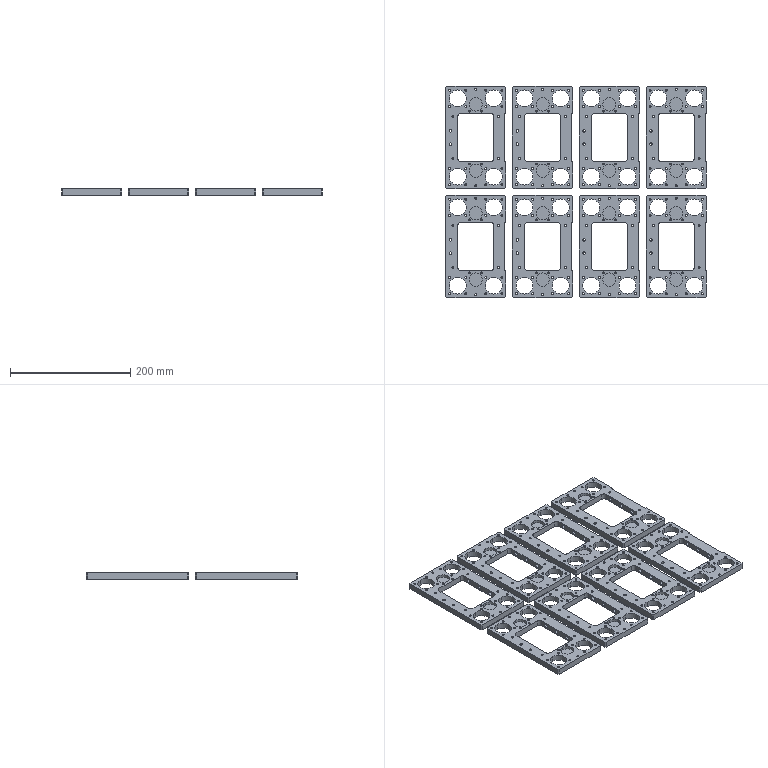CAM job | NX | 3+2 milling, drilling | part box 433 x 351 x 10 mm | stock box 437 x 355 x 10 mm
Tools:
number,name,description,diameter,corner_radius,flute_length,length,flutes
15,D10,Milling Tool-5 Parameters,10.0,0.0,50.0,75.0,2
1,D6A45,Milling Tool-5 Parameters,6.0,0.0,50.0,75.0,2
3,3.3ZT,Drilling Tool,3.3,0.0,35.0,50.0,2
4,4.2ZT,Drilling Tool,4.2,0.0,35.0,50.0,2
14,D10JING,Milling Tool-5 Parameters,10.0,0.0,50.0,75.0,2
10,6.5ZT,Drilling Tool,6.5,0.0,35.0,50.0,2
12,D6,Milling Tool-5 Parameters,6.0,0.0,50.0,75.0,2
Operations:
program,operation,operation_type,tool,method,geometry_group,spindle_rpm,surface_speed,feed_per_tooth,feed_cut,feed_plunge,cut_length_mm,path_length_mm,cut_time_min,machine_time_min
1,DRILLING,Operation,D6A45,METHOD,A,5000.0,94.0,0.035,350.0,0.0,1088.0,8385.885,3.109,3.838
1,DRILLING_COPY,Operation,3.3ZT,METHOD,A,2000.0,20.0,0.05,200.0,0.0,3222.215,11561.448,16.111,16.945
1,DRILLING_COPY_COPY,Operation,4.2ZT,METHOD,A,2000.0,26.0,0.075,300.0,0.0,252.189,1612.278,0.8406,0.9766
1,ZLEVEL_PROFILE,ZLevelMilling,D10,METHOD,A,9500.0,298.0,0.1579,3000.0,1000.0,50422.129,52356.656,17.056,17.25
1,ZLEVEL_PROFILE_COPY,ZLevelMilling,D10,METHOD,A,9500.0,298.0,0.1579,3000.0,1000.0,21441.6,23263.115,7.4,7.583
1,ZLEVEL_PROFILE_COPY_COPY,ZLevelMilling,D10JING,METHOD,A,9500.0,298.0,0.0789,1500.0,1000.0,1943.216,3863.205,1.299,1.491
1,HOLE_MILLING,CylinderMilling,D10JING,METHOD,A,9500.0,298.0,0.1158,2200.0,100.0,43683.929,49403.884,19.856,20.428
1,PLANAR_MILL_COPY_COPY_COPY,PlanarMilling,D6A45,METHOD,A,9500.0,179.0,0.0658,1250.0,100.0,12489.166,35660.013,9.991,12.308
1,ZLEVEL_PROFILE_COPY_1,ZLevelMilling,D10JING,METHOD,A,9500.0,298.0,0.0632,1200.0,1000.0,22980.117,24927.197,19.192,19.386
2,PLANAR_MILL_COPY_COPY_COPY_1,PlanarMilling,D6A45,METHOD,B,9500.0,179.0,0.0658,1250.0,100.0,1424.037,4188.777,1.139,1.416
3,DRILLING_COPY_1,Operation,D6A45,METHOD,C,5000.0,94.0,0.035,350.0,0.0,12.0,144.359,0.0343,0.0475
3,DRILLING_COPY_COPY_COPY,Operation,6.5ZT,METHOD,C,2000.0,26.0,0.075,300.0,0.0,73.358,267.075,0.2445,0.2639
3,刀补,ZLevelMilling,D6,METHOD,C,9500.0,298.0,0.0789,1500.0,1000.0,25.392,223.18,0.0178,0.0376